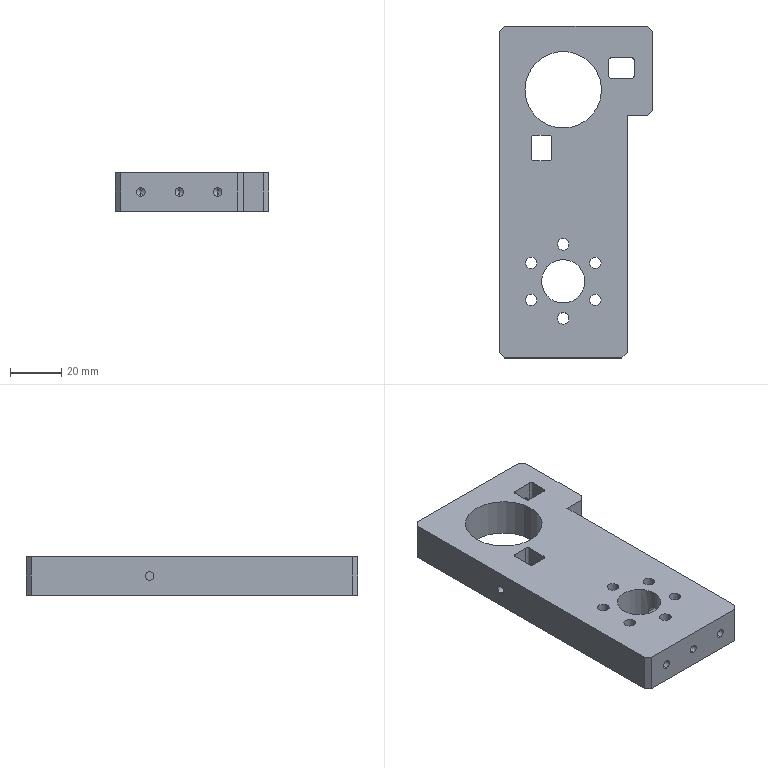Part | STEP file | 05-06 rotary fixing plate | 1 solid | 141 faces | box 60 x 130 x 15 mm | volume 81399 mm3 | cylinder 80 | cone 34 | plane 27 | commonest cylinder face diameters 3.3 x42 4.5 x12 8 x12 2 x8 6 x2 17 x2